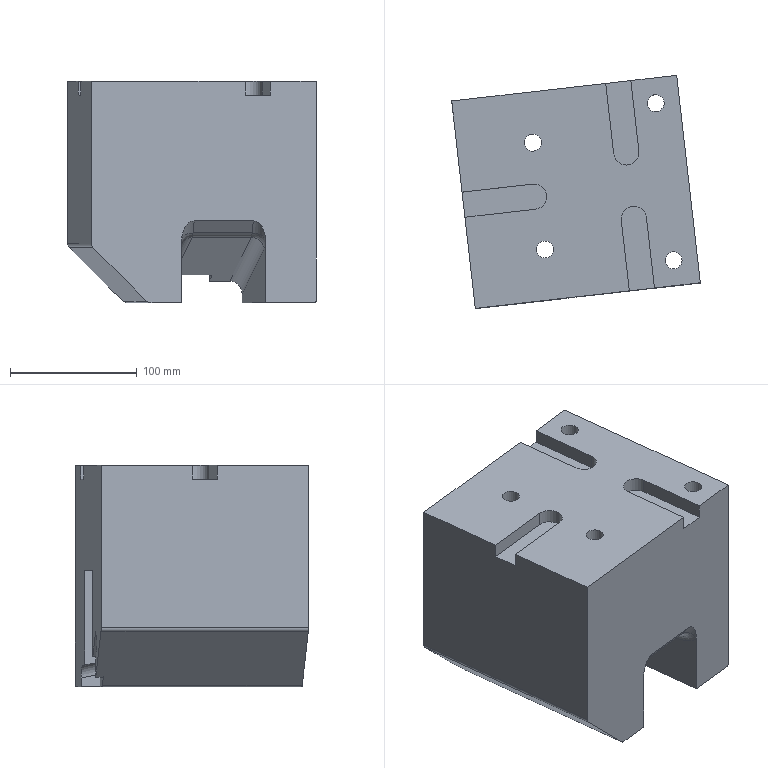Part | NX | features XQ 2 | 1 solid | 64 faces | box 196.528 x 184.203 x 175 mm | volume 4264644 mm3 | plane 34 | cylinder 26 | torus 2 | cone 2 | commonest cylinder face diameters 20 x12 8 x4 13.5 x4 10 x2 10.3 x2 4 x1